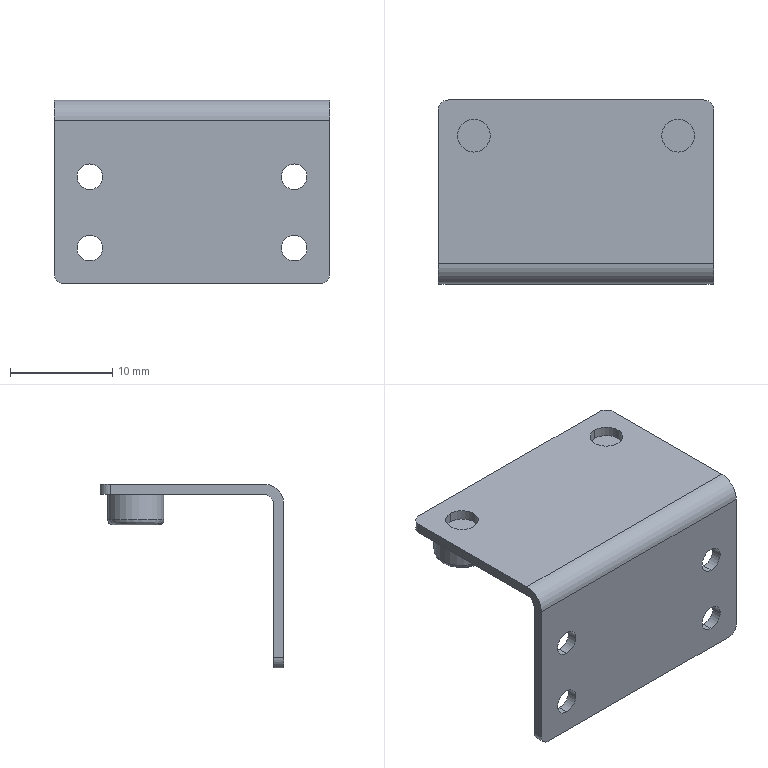Part | SolidWorks | features BaseBody 1 | 1 solid | 52 faces | box 27 x 18 x 18 mm | volume 1018 mm3 | plane 26 | cylinder 22 | spline 4 | commonest cylinder face diameters 2.5 x8 2 x5 3.2 x4 5.5 x4 4 x1